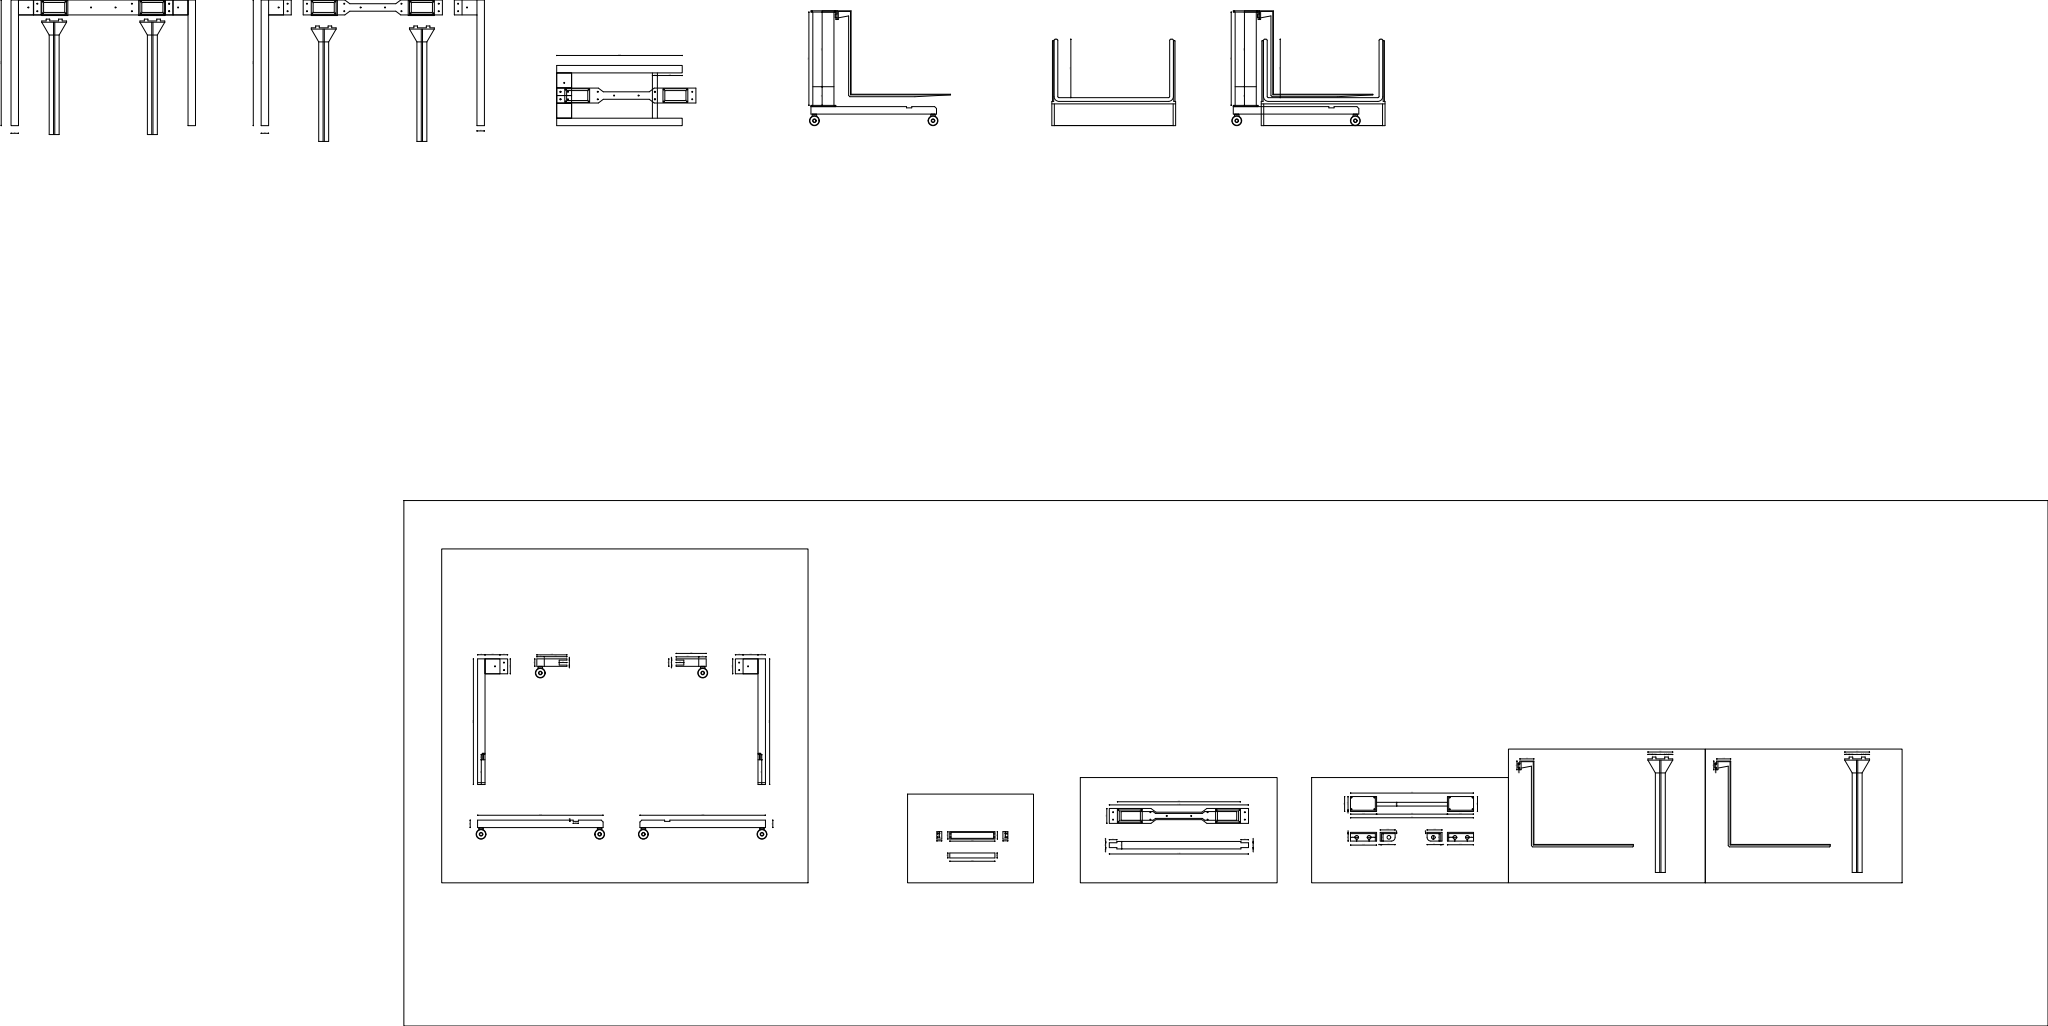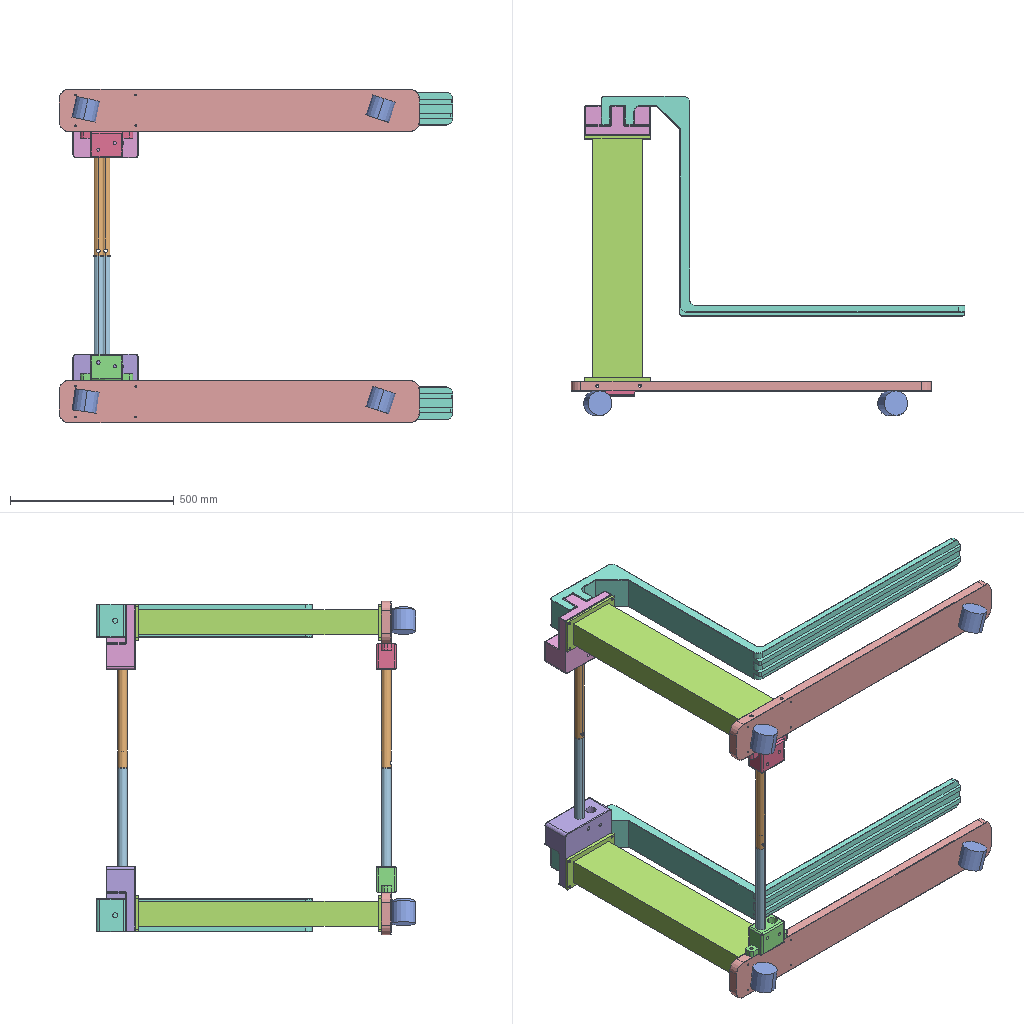Assembly | SolidWorks | 14 different items | 25 placed | box 1202 x 975 x 1019 mm
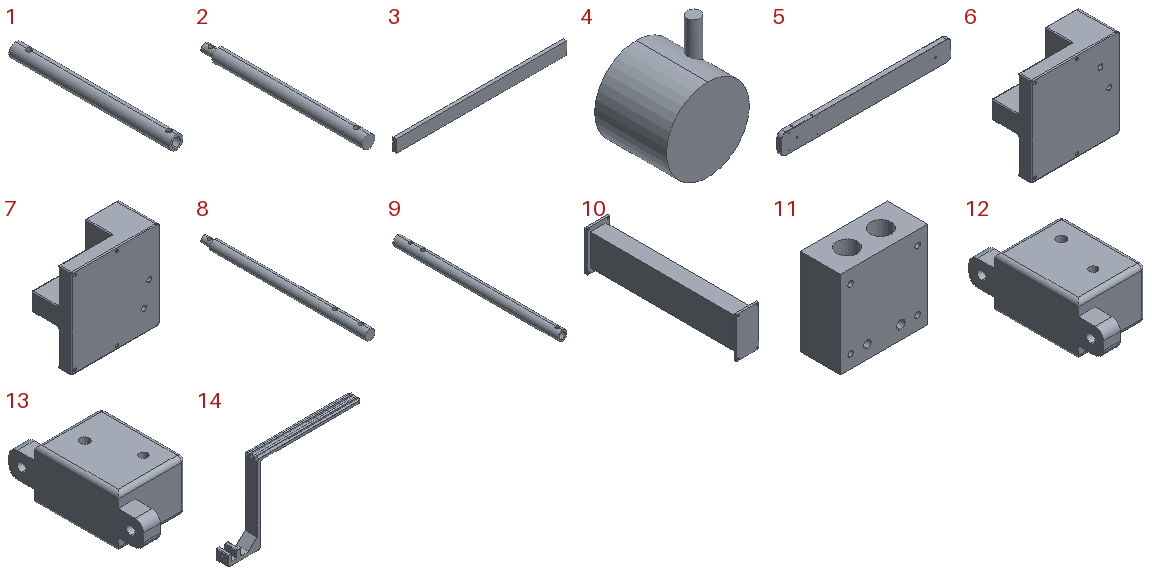Parts list (item | quantity | size | volume | features):
1 | x2 | 30 x 354 x 30 mm | 230741 mm3 | features ICE 2, Extrusion 1, MoveFace 1
2 | x5 | 30 x 384 x 30 mm | 253782 mm3 | features ICE 2, MoveFace 2, Extrusion 1
3 | x1 | 1364 x 30 x 100 mm | 4092000 mm3 | features Extrusion 1
4 | x4 | 75 x 65 x 102.5 mm | 290882 mm3 | features Extrusion 1, ICE 1
5 | x2 | 1100 x 30 x 130 mm | 4243037 mm3 | features HoleWzd 3, Chamfer 1, Extrusion 1, Fillet 1
6 | x1 | 200 x 90 x 200 mm | 2336478 mm3 | features ICE 8, Fillet 2, MoveFace 2, Extrusion 1, HoleWzd 1
7 | x1 | 200 x 90 x 200 mm | 2319927 mm3 | features ICE 7, Fillet 2, Extrusion 1, HoleWzd 1, MoveFace 1
8 | x1 | 30 x 504 x 30 mm | 335802 mm3 | features ICE 3, MoveFace 3, Extrusion 1
9 | x1 | 30 x 514 x 30 mm | 341036 mm3 | features ICE 3, MoveFace 3, Extrusion 1
10 | x2 | 110 x 750 x 200 mm | 9118663 mm3 | features ICE 2, Extrusion 1
11 | x1 | 130 x 60 x 130 mm | 778768 mm3 | features ICE 4, Extrusion 1
12 | x1 | 80 x 160 x 60 mm | 411118 mm3 | features ICE 5, Extrusion 1, Fillet 1
13 | x1 | 80 x 160 x 60 mm | 411118 mm3 | features ICE 5, Extrusion 1, Fillet 1
14 | x2 | 1110 x 100 x 669.85 mm | 5186013 mm3 | features Fillet 6, ICE 3, Chamfer 2, Extrusion 1, MoveFace 1
Mates (type | each side: item.copy, entity, surface, feature):
Coincident | 5.1 face plane Boss-Extrude1 | 10.1 face plane Boss-Extrude1
Concentric | 5.1 face cylinder M6 Tapped Hole1 | 10.1 face cylinder Boss-Extrude1 | 2 times
Concentric | 5.1 face cylinder M12 Tapped Hole1 | 4.1 face cylinder Boss-Extrude2
Tangent | 5.1 face plane Boss-Extrude1 | 4.1 face cylinder Boss-Extrude1
Concentric | 5.1 face cylinder M12 Tapped Hole1 | 4.2 face cylinder Boss-Extrude2
Tangent | 5.1 face plane Boss-Extrude1 | 4.2 face cylinder Boss-Extrude1
Concentric | 5.2 face cylinder M6 Tapped Hole1 | 10.2 face cylinder Boss-Extrude1 | 2 times
Concentric | 5.2 face cylinder M12 Tapped Hole1 | 4.3 face cylinder Boss-Extrude2
Concentric | 5.2 face cylinder M12 Tapped Hole1 | 4.4 face cylinder Boss-Extrude2
Tangent | 5.2 face plane Boss-Extrude1 | 4.3 face cylinder Boss-Extrude1
Coincident | 5.2 face plane Boss-Extrude1 | 10.2 face plane Boss-Extrude1
Tangent | 5.2 face plane Boss-Extrude1 | 4.4 face cylinder Boss-Extrude1
Coincident | 5.1 face plane Boss-Extrude1 | 5.2 face plane Boss-Extrude1 | 2 times
Coincident | 10.1 face plane Boss-Extrude4 | 6.1 face plane Boss-Extrude1 | 3 times
Concentric | 1.1 face cylinder Boss-Extrude1 | 6.1 face cylinder Cut-Extrude1
Concentric | 6.1 face cylinder Cut-Extrude2 | 1.1 face cylinder Cut-Extrude3
Concentric | 1.1 face cylinder Boss-Extrude1 | 2.1 face cylinder Boss-Extrude1
Coincident | 10.2 face plane Boss-Extrude4 | 7.1 face plane Boss-Extrude1 | 3 times
Concentric | 6.1 face cylinder Cut-Extrude3 | 2.2 face cylinder Boss-Extrude1
Concentric | 6.1 face cylinder Cut-Extrude5 | 2.2 face cylinder Cut-Extrude1
Coincident | 14.1 face plane Boss-Extrude1 | 7.1 face plane Boss-Extrude2
Coincident | 6.1 face plane Boss-Extrude2 | 14.2 face plane Boss-Extrude1
DistanceDim | 14.2 face plane Boss-Extrude1 | 6.1 face plane Boss-Extrude2
Coincident | 6.1 face plane Boss-Extrude1 | 14.2 face plane Boss-Extrude1
Coincident | 14.1 face plane Boss-Extrude1 | 7.1 face plane Boss-Extrude1
DistanceDim | 14.1 face plane Boss-Extrude1 | 7.1 face plane Boss-Extrude2
Coincident | 5.1 face plane Boss-Extrude1 | 13.1 face plane Boss-Extrude1
Concentric | 5.1 face cylinder M10 Tapped Hole1 | 13.1 face cylinder Boss-Extrude2 | 2 times
Coincident | 5.2 face plane Boss-Extrude1 | 12.1 face plane Boss-Extrude1
Concentric | 5.2 face cylinder M10 Tapped Hole1 | 12.1 face cylinder Boss-Extrude2 | 2 times
Concentric | 13.1 face cylinder Cut-Extrude1 | 1.2 face cylinder Boss-Extrude1
Concentric | 13.1 face cylinder Cut-Extrude1 | 2.3 face cylinder Boss-Extrude1
Concentric | 13.1 face cylinder Cut-Extrude3 | 2.3 face cylinder Cut-Extrude1
Concentric | 7.1 face cylinder Cut-Extrude1 | 2.4 face cylinder Boss-Extrude1
Concentric | 1.1 face cylinder Cut-Extrude3 | 2.4 face cylinder Cut-Extrude1
Concentric | 13.1 face cylinder Cut-Extrude3 | 1.2 face cylinder Cut-Extrude3
Concentric | 1.2 face cylinder Boss-Extrude1 | 2.5 face cylinder Boss-Extrude1
Concentric | 1.2 face cylinder Cut-Extrude3 | 2.5 face cylinder Cut-Extrude1